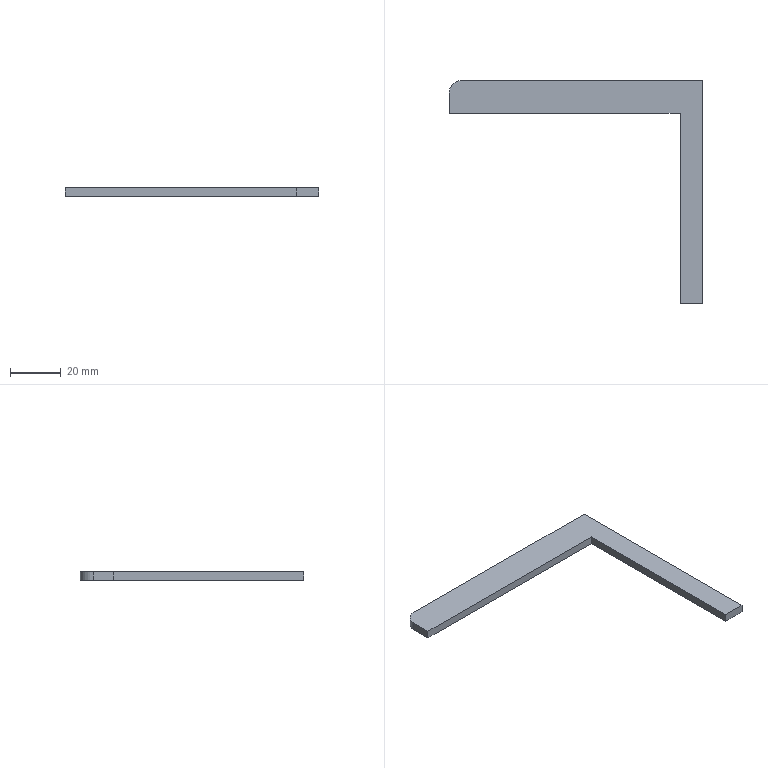Part | SolidWorks | features FlatPattern 1, SMBaseFlange 1, SheetMetal 1 | 1 solid | 9 faces | box 100 x 88 x 3.2 mm | volume 6303 mm3 | plane 8 | cylinder 1 | commonest cylinder face diameters 10 x1
STEP:
#1=CARTESIAN_POINT('',(100.,4.,0.));
#2=VERTEX_POINT('',#1);
#3=CARTESIAN_POINT('',(100.,92.,0.));
#4=VERTEX_POINT('',#3);
#5=CARTESIAN_POINT('',(100.,92.,0.));
#6=DIRECTION('',(0.,1.,0.));
#7=VECTOR('',#6,1000.);
#8=LINE('',#5,#7);
#9=EDGE_CURVE('',#2,#4,#8,.T.);
#10=ORIENTED_EDGE('',*,*,#9,.T.);
#11=CARTESIAN_POINT('',(100.,92.,3.2));
#12=VERTEX_POINT('',#11);
#13=CARTESIAN_POINT('',(100.,92.,3.2));
#14=DIRECTION('',(0.,0.,-1.));
#15=VECTOR('',#14,1000.);
#16=LINE('',#13,#15);
#17=EDGE_CURVE('',#12,#4,#16,.T.);
#18=ORIENTED_EDGE('',*,*,#17,.F.);
#19=CARTESIAN_POINT('',(100.,4.,3.2));
#20=VERTEX_POINT('',#19);
#21=CARTESIAN_POINT('',(100.,92.,3.2));
#22=DIRECTION('',(0.,1.,0.));
#23=VECTOR('',#22,1000.);
#24=LINE('',#21,#23);
#25=EDGE_CURVE('',#20,#12,#24,.T.);
#26=ORIENTED_EDGE('',*,*,#25,.F.);
#27=CARTESIAN_POINT('',(100.,4.,3.2));
#28=DIRECTION('',(0.,0.,-1.));
#29=VECTOR('',#28,1000.);
#30=LINE('',#27,#29);
#31=EDGE_CURVE('',#20,#2,#30,.T.);
#32=ORIENTED_EDGE('',*,*,#31,.T.);
#33=EDGE_LOOP('',(#10,#18,#26,#32));
#34=FACE_OUTER_BOUND('',#33,.T.);
#35=CARTESIAN_POINT('',(100.,92.,3.2));
#36=DIRECTION('',(-1.,0.,0.));
#37=DIRECTION('',(0.,-1.,0.));
#38=AXIS2_PLACEMENT_3D('',#35,#36,#37);
#39=PLANE('',#38);
#40=ADVANCED_FACE('',(#34),#39,.F.);
#41=CARTESIAN_POINT('',(5.,92.,0.));
#42=VERTEX_POINT('',#41);
#43=CARTESIAN_POINT('',(5.,92.,0.));
#44=DIRECTION('',(-1.,0.,0.));
#45=VECTOR('',#44,1000.);
#46=LINE('',#43,#45);
#47=EDGE_CURVE('',#4,#42,#46,.T.);
#48=ORIENTED_EDGE('',*,*,#47,.T.);
#49=CARTESIAN_POINT('',(5.,92.,3.2));
#50=VERTEX_POINT('',#49);
#51=CARTESIAN_POINT('',(5.,92.,3.2));
#52=DIRECTION('',(0.,0.,-1.));
#53=VECTOR('',#52,1000.);
#54=LINE('',#51,#53);
#55=EDGE_CURVE('',#50,#42,#54,.T.);
#56=ORIENTED_EDGE('',*,*,#55,.F.);
#57=CARTESIAN_POINT('',(5.,92.,3.2));
#58=DIRECTION('',(-1.,0.,0.));
#59=VECTOR('',#58,1000.);
#60=LINE('',#57,#59);
#61=EDGE_CURVE('',#12,#50,#60,.T.);
#62=ORIENTED_EDGE('',*,*,#61,.F.);
#63=ORIENTED_EDGE('',*,*,#17,.T.);
#64=EDGE_LOOP('',(#48,#56,#62,#63));
#65=FACE_OUTER_BOUND('',#64,.T.);
#66=CARTESIAN_POINT('',(5.,92.,3.2));
#67=DIRECTION('',(0.,-1.,0.));
#68=DIRECTION('',(0.,0.,-1.));
#69=AXIS2_PLACEMENT_3D('',#66,#67,#68);
#70=PLANE('',#69);
#71=ADVANCED_FACE('',(#65),#70,.F.);
#72=CARTESIAN_POINT('',(0.,87.,0.));
#73=VERTEX_POINT('',#72);
#74=CARTESIAN_POINT('',(5.,87.,0.));
#75=DIRECTION('',(0.,0.,1.));
#76=DIRECTION('',(-1.,0.,0.));
#77=AXIS2_PLACEMENT_3D('',#74,#75,#76);
#78=CIRCLE('',#77,5.);
#79=EDGE_CURVE('',#42,#73,#78,.T.);
#80=ORIENTED_EDGE('',*,*,#79,.T.);
#81=CARTESIAN_POINT('',(0.,87.,3.2));
#82=VERTEX_POINT('',#81);
#83=CARTESIAN_POINT('',(0.,87.,3.2));
#84=DIRECTION('',(0.,0.,-1.));
#85=VECTOR('',#84,1000.);
#86=LINE('',#83,#85);
#87=EDGE_CURVE('',#82,#73,#86,.T.);
#88=ORIENTED_EDGE('',*,*,#87,.F.);
#89=CARTESIAN_POINT('',(5.,87.,3.2));
#90=DIRECTION('',(0.,0.,1.));
#91=DIRECTION('',(-1.,0.,0.));
#92=AXIS2_PLACEMENT_3D('',#89,#90,#91);
#93=CIRCLE('',#92,5.);
#94=EDGE_CURVE('',#50,#82,#93,.T.);
#95=ORIENTED_EDGE('',*,*,#94,.F.);
#96=ORIENTED_EDGE('',*,*,#55,.T.);
#97=EDGE_LOOP('',(#80,#88,#95,#96));
#98=FACE_OUTER_BOUND('',#97,.T.);
#99=CARTESIAN_POINT('',(5.,87.,3.2));
#100=DIRECTION('',(0.,0.,-1.));
#101=DIRECTION('',(-1.,0.,0.));
#102=AXIS2_PLACEMENT_3D('',#99,#100,#101);
#103=CYLINDRICAL_SURFACE('',#102,5.);
#104=ADVANCED_FACE('',(#98),#103,.T.);
#105=CARTESIAN_POINT('',(0.,79.,0.));
#106=VERTEX_POINT('',#105);
#107=CARTESIAN_POINT('',(0.,79.,0.));
#108=DIRECTION('',(0.,-1.,0.));
#109=VECTOR('',#108,1000.);
#110=LINE('',#107,#109);
#111=EDGE_CURVE('',#73,#106,#110,.T.);
#112=ORIENTED_EDGE('',*,*,#111,.T.);
#113=CARTESIAN_POINT('',(0.,79.,3.2));
#114=VERTEX_POINT('',#113);
#115=CARTESIAN_POINT('',(0.,79.,3.2));
#116=DIRECTION('',(0.,0.,-1.));
#117=VECTOR('',#116,1000.);
#118=LINE('',#115,#117);
#119=EDGE_CURVE('',#114,#106,#118,.T.);
#120=ORIENTED_EDGE('',*,*,#119,.F.);
#121=CARTESIAN_POINT('',(0.,79.,3.2));
#122=DIRECTION('',(0.,-1.,0.));
#123=VECTOR('',#122,1000.);
#124=LINE('',#121,#123);
#125=EDGE_CURVE('',#82,#114,#124,.T.);
#126=ORIENTED_EDGE('',*,*,#125,.F.);
#127=ORIENTED_EDGE('',*,*,#87,.T.);
#128=EDGE_LOOP('',(#112,#120,#126,#127));
#129=FACE_OUTER_BOUND('',#128,.T.);
#130=CARTESIAN_POINT('',(0.,79.,3.2));
#131=DIRECTION('',(1.,0.,0.));
#132=DIRECTION('',(0.,0.,-1.));
#133=AXIS2_PLACEMENT_3D('',#130,#131,#132);
#134=PLANE('',#133);
#135=ADVANCED_FACE('',(#129),#134,.F.);
#136=CARTESIAN_POINT('',(91.,79.,0.));
#137=VERTEX_POINT('',#136);
#138=CARTESIAN_POINT('',(91.,79.,0.));
#139=DIRECTION('',(1.,0.,0.));
#140=VECTOR('',#139,1000.);
#141=LINE('',#138,#140);
#142=EDGE_CURVE('',#106,#137,#141,.T.);
#143=ORIENTED_EDGE('',*,*,#142,.T.);
#144=CARTESIAN_POINT('',(91.,79.,3.2));
#145=VERTEX_POINT('',#144);
#146=CARTESIAN_POINT('',(91.,79.,3.2));
#147=DIRECTION('',(0.,0.,-1.));
#148=VECTOR('',#147,1000.);
#149=LINE('',#146,#148);
#150=EDGE_CURVE('',#145,#137,#149,.T.);
#151=ORIENTED_EDGE('',*,*,#150,.F.);
#152=CARTESIAN_POINT('',(91.,79.,3.2));
#153=DIRECTION('',(1.,0.,0.));
#154=VECTOR('',#153,1000.);
#155=LINE('',#152,#154);
#156=EDGE_CURVE('',#114,#145,#155,.T.);
#157=ORIENTED_EDGE('',*,*,#156,.F.);
#158=ORIENTED_EDGE('',*,*,#119,.T.);
#159=EDGE_LOOP('',(#143,#151,#157,#158));
#160=FACE_OUTER_BOUND('',#159,.T.);
#161=CARTESIAN_POINT('',(91.,79.,3.2));
#162=DIRECTION('',(0.,1.,0.));
#163=DIRECTION('',(-1.,0.,0.));
#164=AXIS2_PLACEMENT_3D('',#161,#162,#163);
#165=PLANE('',#164);
#166=ADVANCED_FACE('',(#160),#165,.F.);
#167=CARTESIAN_POINT('',(91.,4.,0.));
#168=VERTEX_POINT('',#167);
#169=CARTESIAN_POINT('',(91.,4.,0.));
#170=DIRECTION('',(0.,-1.,0.));
#171=VECTOR('',#170,1000.);
#172=LINE('',#169,#171);
#173=EDGE_CURVE('',#137,#168,#172,.T.);
#174=ORIENTED_EDGE('',*,*,#173,.T.);
#175=CARTESIAN_POINT('',(91.,4.,3.2));
#176=VERTEX_POINT('',#175);
#177=CARTESIAN_POINT('',(91.,4.,3.2));
#178=DIRECTION('',(0.,0.,-1.));
#179=VECTOR('',#178,1000.);
#180=LINE('',#177,#179);
#181=EDGE_CURVE('',#176,#168,#180,.T.);
#182=ORIENTED_EDGE('',*,*,#181,.F.);
#183=CARTESIAN_POINT('',(91.,4.,3.2));
#184=DIRECTION('',(0.,-1.,0.));
#185=VECTOR('',#184,1000.);
#186=LINE('',#183,#185);
#187=EDGE_CURVE('',#145,#176,#186,.T.);
#188=ORIENTED_EDGE('',*,*,#187,.F.);
#189=ORIENTED_EDGE('',*,*,#150,.T.);
#190=EDGE_LOOP('',(#174,#182,#188,#189));
#191=FACE_OUTER_BOUND('',#190,.T.);
#192=CARTESIAN_POINT('',(91.,4.,3.2));
#193=DIRECTION('',(1.,0.,0.));
#194=DIRECTION('',(0.,0.,-1.));
#195=AXIS2_PLACEMENT_3D('',#192,#193,#194);
#196=PLANE('',#195);
#197=ADVANCED_FACE('',(#191),#196,.F.);
#198=CARTESIAN_POINT('',(100.,4.,0.));
#199=DIRECTION('',(1.,0.,0.));
#200=VECTOR('',#199,1000.);
#201=LINE('',#198,#200);
#202=EDGE_CURVE('',#168,#2,#201,.T.);
#203=ORIENTED_EDGE('',*,*,#202,.T.);
#204=ORIENTED_EDGE('',*,*,#31,.F.);
#205=CARTESIAN_POINT('',(100.,4.,3.2));
#206=DIRECTION('',(1.,0.,0.));
#207=VECTOR('',#206,1000.);
#208=LINE('',#205,#207);
#209=EDGE_CURVE('',#176,#20,#208,.T.);
#210=ORIENTED_EDGE('',*,*,#209,.F.);
#211=ORIENTED_EDGE('',*,*,#181,.T.);
#212=EDGE_LOOP('',(#203,#204,#210,#211));
#213=FACE_OUTER_BOUND('',#212,.T.);
#214=CARTESIAN_POINT('',(100.,4.,3.2));
#215=DIRECTION('',(0.,1.,0.));
#216=DIRECTION('',(-1.,0.,0.));
#217=AXIS2_PLACEMENT_3D('',#214,#215,#216);
#218=PLANE('',#217);
#219=ADVANCED_FACE('',(#213),#218,.F.);
#220=ORIENTED_EDGE('',*,*,#25,.T.);
#221=ORIENTED_EDGE('',*,*,#61,.T.);
#222=ORIENTED_EDGE('',*,*,#94,.T.);
#223=ORIENTED_EDGE('',*,*,#125,.T.);
#224=ORIENTED_EDGE('',*,*,#156,.T.);
#225=ORIENTED_EDGE('',*,*,#187,.T.);
#226=ORIENTED_EDGE('',*,*,#209,.T.);
#227=EDGE_LOOP('',(#220,#221,#222,#223,#224,#225,#226));
#228=FACE_OUTER_BOUND('',#227,.T.);
#229=CARTESIAN_POINT('',(5.,87.,3.2));
#230=DIRECTION('',(0.,0.,-1.));
#231=DIRECTION('',(-1.,0.,0.));
#232=AXIS2_PLACEMENT_3D('',#229,#230,#231);
#233=PLANE('',#232);
#234=ADVANCED_FACE('',(#228),#233,.F.);
#235=ORIENTED_EDGE('',*,*,#9,.F.);
#236=ORIENTED_EDGE('',*,*,#202,.F.);
#237=ORIENTED_EDGE('',*,*,#173,.F.);
#238=ORIENTED_EDGE('',*,*,#142,.F.);
#239=ORIENTED_EDGE('',*,*,#111,.F.);
#240=ORIENTED_EDGE('',*,*,#79,.F.);
#241=ORIENTED_EDGE('',*,*,#47,.F.);
#242=EDGE_LOOP('',(#235,#236,#237,#238,#239,#240,#241));
#243=FACE_OUTER_BOUND('',#242,.T.);
#244=CARTESIAN_POINT('',(5.,87.,0.));
#245=DIRECTION('',(0.,0.,-1.));
#246=DIRECTION('',(-1.,0.,0.));
#247=AXIS2_PLACEMENT_3D('',#244,#245,#246);
#248=PLANE('',#247);
#249=ADVANCED_FACE('',(#243),#248,.T.);
#250=CLOSED_SHELL('',(#40,#71,#104,#135,#166,#197,#219,#234,#249));
#251=MANIFOLD_SOLID_BREP('',#250);
#252=CARTESIAN_POINT('',(0.,0.,0.));
#253=DIRECTION('',(0.,0.,1.));
#254=DIRECTION('',(1.,0.,0.));
#255=AXIS2_PLACEMENT_3D('',#252,#253,#254);
#256=(LENGTH_UNIT()NAMED_UNIT(*)SI_UNIT(.MILLI.,.METRE.));
#257=UNCERTAINTY_MEASURE_WITH_UNIT(LENGTH_MEASURE(0.00001),#256,'','');
#258=(NAMED_UNIT(*)PLANE_ANGLE_UNIT()SI_UNIT($,.RADIAN.));
#259=(NAMED_UNIT(*)SI_UNIT($,.STERADIAN.)SOLID_ANGLE_UNIT());
#260=(GEOMETRIC_REPRESENTATION_CONTEXT(3)GLOBAL_UNCERTAINTY_ASSIGNED_CONTEXT((#257))GLOBAL_UNIT_ASSIGNED_CONTEXT((#256,#258,#259))REPRESENTATION_CONTEXT('',''));
#261=ADVANCED_BREP_SHAPE_REPRESENTATION('',(#251,#255),#260);